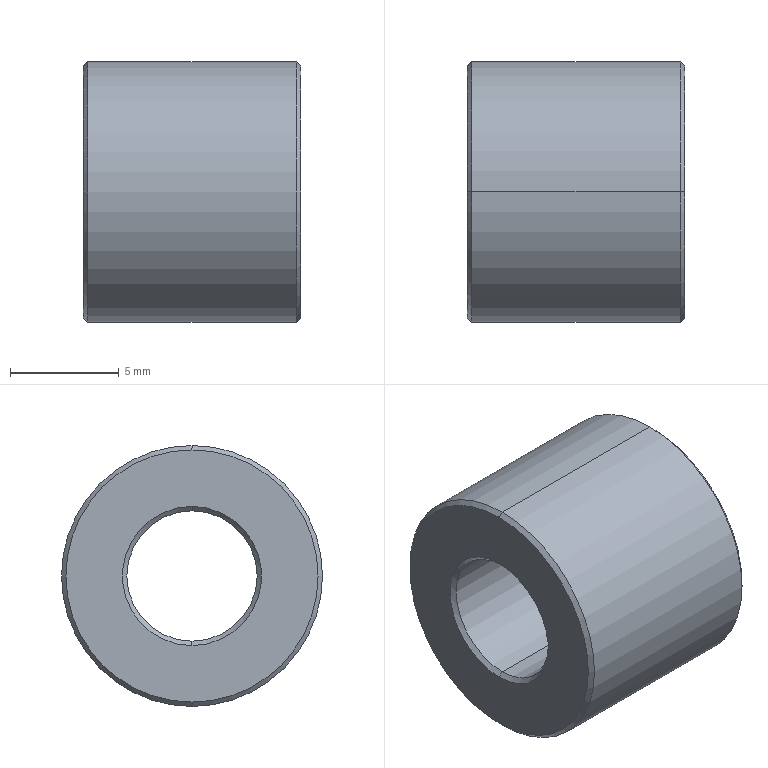Part | STEP file | KNCLM6-12-10 | 1 solid | 14 faces | box 10 x 12 x 12 mm | volume 845.968 mm3 | cone 8 | cylinder 4 | plane 2 | commonest cylinder face diameters 6 x2 12 x2
STEP:
#1=CARTESIAN_POINT('',(0.,0.,0.));
#2=DIRECTION('',(0.,0.,1.));
#3=DIRECTION('',(1.,0.,0.));
#4=AXIS2_PLACEMENT_3D('',#1,#2,#3);
#5=CARTESIAN_POINT('',(10.,0.,-5.8));
#6=VERTEX_POINT('',#5);
#7=CARTESIAN_POINT('',(10.,0.,5.8));
#8=VERTEX_POINT('',#7);
#9=CARTESIAN_POINT('',(10.,0.,0.));
#10=DIRECTION('',(1.,0.,0.));
#11=DIRECTION('',(0.,0.,1.));
#12=AXIS2_PLACEMENT_3D('',#9,#10,#11);
#13=CIRCLE('',#12,5.8);
#14=CARTESIAN_POINT('',(9.8,0.,0.));
#15=DIRECTION('',(-1.,0.,0.));
#16=DIRECTION('',(0.,0.,1.));
#17=AXIS2_PLACEMENT_3D('',#14,#15,#16);
#18=CONICAL_SURFACE('',#17,6.,0.7854);
#19=CARTESIAN_POINT('',(6.283,-0.2));
#20=DIRECTION('',(-1.,0.));
#21=VECTOR('',#20,1.);
#22=LINE('',#19,#21);
#23=(GEOMETRIC_REPRESENTATION_CONTEXT(2)PARAMETRIC_REPRESENTATION_CONTEXT()REPRESENTATION_CONTEXT('',''));
#24=DEFINITIONAL_REPRESENTATION('',(#22),#23);
#25=PCURVE('',#18,#24);
#26=CARTESIAN_POINT('',(10.,3.,0.));
#27=DIRECTION('',(-1.,0.,0.));
#28=DIRECTION('',(0.,0.,1.));
#29=AXIS2_PLACEMENT_3D('',#26,#27,#28);
#30=PLANE('',#29);
#31=CARTESIAN_POINT('',(5.8,-3.));
#32=CARTESIAN_POINT('',(5.8,-13.046));
#33=CARTESIAN_POINT('',(-2.9,-8.023));
#34=CARTESIAN_POINT('',(-11.6,-3.));
#35=CARTESIAN_POINT('',(-2.9,2.023));
#36=CARTESIAN_POINT('',(5.8,7.046));
#37=CARTESIAN_POINT('',(5.8,-3.));
#38=(BOUNDED_CURVE()B_SPLINE_CURVE(2,(#31,#32,#33,#34,#35,#36,#37),.UNSPECIFIED.,.T.,.F.)B_SPLINE_CURVE_WITH_KNOTS((1,2,2,2,2,1),(-2.094,0.,2.094,4.189,6.283,8.378),.UNSPECIFIED.)CURVE()GEOMETRIC_REPRESENTATION_ITEM()RATIONAL_B_SPLINE_CURVE((1.,0.5,1.,0.5,1.,0.5,1.))REPRESENTATION_ITEM(''));
#39=(GEOMETRIC_REPRESENTATION_CONTEXT(2)PARAMETRIC_REPRESENTATION_CONTEXT()REPRESENTATION_CONTEXT('',''));
#40=DEFINITIONAL_REPRESENTATION('',(#38),#39);
#41=PCURVE('',#30,#40);
#42=SURFACE_CURVE('',#13,(#25,#41),.PCURVE_S1.);
#43=EDGE_CURVE('',#6,#8,#42,.T.);
#44=ORIENTED_EDGE('',*,*,#43,.F.);
#45=CARTESIAN_POINT('',(9.8,0.,-6.));
#46=VERTEX_POINT('',#45);
#47=CARTESIAN_POINT('',(9.8,0.,-6.));
#48=DIRECTION('',(-0.7071,0.,-0.7071));
#49=VECTOR('',#48,1.);
#50=LINE('',#47,#49);
#51=CARTESIAN_POINT('',(3.142,0.));
#52=DIRECTION('',(0.,1.));
#53=VECTOR('',#52,1.);
#54=LINE('',#51,#53);
#55=(GEOMETRIC_REPRESENTATION_CONTEXT(2)PARAMETRIC_REPRESENTATION_CONTEXT()REPRESENTATION_CONTEXT('',''));
#56=DEFINITIONAL_REPRESENTATION('',(#54),#55);
#57=PCURVE('',#18,#56);
#58=CARTESIAN_POINT('',(9.8,0.,0.));
#59=DIRECTION('',(-1.,0.,0.));
#60=DIRECTION('',(0.,0.,1.));
#61=AXIS2_PLACEMENT_3D('',#58,#59,#60);
#62=CONICAL_SURFACE('',#61,6.,0.7854);
#63=CARTESIAN_POINT('',(3.142,0.));
#64=DIRECTION('',(0.,1.));
#65=VECTOR('',#64,1.);
#66=LINE('',#63,#65);
#67=(GEOMETRIC_REPRESENTATION_CONTEXT(2)PARAMETRIC_REPRESENTATION_CONTEXT()REPRESENTATION_CONTEXT('',''));
#68=DEFINITIONAL_REPRESENTATION('',(#66),#67);
#69=PCURVE('',#62,#68);
#70=SURFACE_CURVE('',#50,(#57,#69),.PCURVE_S1.);
#71=EDGE_CURVE('',#6,#46,#70,.T.);
#72=ORIENTED_EDGE('',*,*,#71,.T.);
#73=CARTESIAN_POINT('',(9.8,0.,6.));
#74=VERTEX_POINT('',#73);
#75=CARTESIAN_POINT('',(9.8,0.,0.));
#76=DIRECTION('',(-1.,0.,0.));
#77=DIRECTION('',(0.,0.,1.));
#78=AXIS2_PLACEMENT_3D('',#75,#76,#77);
#79=CIRCLE('',#78,6.);
#80=CARTESIAN_POINT('',(0.,0.));
#81=DIRECTION('',(1.,0.));
#82=VECTOR('',#81,1.);
#83=LINE('',#80,#82);
#84=(GEOMETRIC_REPRESENTATION_CONTEXT(2)PARAMETRIC_REPRESENTATION_CONTEXT()REPRESENTATION_CONTEXT('',''));
#85=DEFINITIONAL_REPRESENTATION('',(#83),#84);
#86=PCURVE('',#18,#85);
#87=CARTESIAN_POINT('',(0.,0.,0.));
#88=DIRECTION('',(-1.,0.,0.));
#89=DIRECTION('',(0.,0.,1.));
#90=AXIS2_PLACEMENT_3D('',#87,#88,#89);
#91=CYLINDRICAL_SURFACE('',#90,6.);
#92=CARTESIAN_POINT('',(0.,-9.8));
#93=DIRECTION('',(1.,0.));
#94=VECTOR('',#93,1.);
#95=LINE('',#92,#94);
#96=(GEOMETRIC_REPRESENTATION_CONTEXT(2)PARAMETRIC_REPRESENTATION_CONTEXT()REPRESENTATION_CONTEXT('',''));
#97=DEFINITIONAL_REPRESENTATION('',(#95),#96);
#98=PCURVE('',#91,#97);
#99=SURFACE_CURVE('',#79,(#86,#98),.PCURVE_S1.);
#100=EDGE_CURVE('',#74,#46,#99,.T.);
#101=ORIENTED_EDGE('',*,*,#100,.F.);
#102=CARTESIAN_POINT('',(9.8,0.,6.));
#103=DIRECTION('',(-0.7071,0.,0.7071));
#104=VECTOR('',#103,1.);
#105=LINE('',#102,#104);
#106=CARTESIAN_POINT('',(0.,0.));
#107=DIRECTION('',(0.,1.));
#108=VECTOR('',#107,1.);
#109=LINE('',#106,#108);
#110=(GEOMETRIC_REPRESENTATION_CONTEXT(2)PARAMETRIC_REPRESENTATION_CONTEXT()REPRESENTATION_CONTEXT('',''));
#111=DEFINITIONAL_REPRESENTATION('',(#109),#110);
#112=PCURVE('',#18,#111);
#113=CARTESIAN_POINT('',(6.283,0.));
#114=DIRECTION('',(0.,1.));
#115=VECTOR('',#114,1.);
#116=LINE('',#113,#115);
#117=(GEOMETRIC_REPRESENTATION_CONTEXT(2)PARAMETRIC_REPRESENTATION_CONTEXT()REPRESENTATION_CONTEXT('',''));
#118=DEFINITIONAL_REPRESENTATION('',(#116),#117);
#119=PCURVE('',#62,#118);
#120=SURFACE_CURVE('',#105,(#112,#119),.PCURVE_S1.);
#121=EDGE_CURVE('',#8,#74,#120,.T.);
#122=ORIENTED_EDGE('',*,*,#121,.F.);
#123=EDGE_LOOP('',(#44,#72,#101,#122));
#124=FACE_BOUND('',#123,.T.);
#125=ADVANCED_FACE('',(#124),#18,.T.);
#126=CARTESIAN_POINT('',(9.8,0.,-3.));
#127=VERTEX_POINT('',#126);
#128=CARTESIAN_POINT('',(10.,0.,-3.2));
#129=VERTEX_POINT('',#128);
#130=CARTESIAN_POINT('',(10.,0.,-3.2));
#131=DIRECTION('',(0.7071,0.,-0.7071));
#132=VECTOR('',#131,1.);
#133=LINE('',#130,#132);
#134=CARTESIAN_POINT('',(10.,0.,0.));
#135=DIRECTION('',(1.,0.,0.));
#136=DIRECTION('',(0.,0.,-1.));
#137=AXIS2_PLACEMENT_3D('',#134,#135,#136);
#138=CONICAL_SURFACE('',#137,3.2,0.7854);
#139=CARTESIAN_POINT('',(6.283,0.));
#140=DIRECTION('',(0.,1.));
#141=VECTOR('',#140,1.);
#142=LINE('',#139,#141);
#143=(GEOMETRIC_REPRESENTATION_CONTEXT(2)PARAMETRIC_REPRESENTATION_CONTEXT()REPRESENTATION_CONTEXT('',''));
#144=DEFINITIONAL_REPRESENTATION('',(#142),#143);
#145=PCURVE('',#138,#144);
#146=CARTESIAN_POINT('',(10.,0.,0.));
#147=DIRECTION('',(1.,0.,0.));
#148=DIRECTION('',(0.,0.,-1.));
#149=AXIS2_PLACEMENT_3D('',#146,#147,#148);
#150=CONICAL_SURFACE('',#149,3.2,0.7854);
#151=CARTESIAN_POINT('',(0.,0.));
#152=DIRECTION('',(0.,1.));
#153=VECTOR('',#152,1.);
#154=LINE('',#151,#153);
#155=(GEOMETRIC_REPRESENTATION_CONTEXT(2)PARAMETRIC_REPRESENTATION_CONTEXT()REPRESENTATION_CONTEXT('',''));
#156=DEFINITIONAL_REPRESENTATION('',(#154),#155);
#157=PCURVE('',#150,#156);
#158=SURFACE_CURVE('',#133,(#145,#157),.PCURVE_S1.);
#159=EDGE_CURVE('',#127,#129,#158,.T.);
#160=ORIENTED_EDGE('',*,*,#159,.T.);
#161=CARTESIAN_POINT('',(10.,0.,3.2));
#162=VERTEX_POINT('',#161);
#163=CARTESIAN_POINT('',(10.,0.,0.));
#164=DIRECTION('',(-1.,0.,0.));
#165=DIRECTION('',(0.,0.,1.));
#166=AXIS2_PLACEMENT_3D('',#163,#164,#165);
#167=CIRCLE('',#166,3.2);
#168=CARTESIAN_POINT('',(9.425,0.));
#169=DIRECTION('',(-1.,0.));
#170=VECTOR('',#169,1.);
#171=LINE('',#168,#170);
#172=(GEOMETRIC_REPRESENTATION_CONTEXT(2)PARAMETRIC_REPRESENTATION_CONTEXT()REPRESENTATION_CONTEXT('',''));
#173=DEFINITIONAL_REPRESENTATION('',(#171),#172);
#174=PCURVE('',#138,#173);
#175=CARTESIAN_POINT('',(0.,-3.));
#176=DIRECTION('',(1.,0.));
#177=AXIS2_PLACEMENT_2D('',#175,#176);
#178=CIRCLE('',#177,3.2);
#179=(GEOMETRIC_REPRESENTATION_CONTEXT(2)PARAMETRIC_REPRESENTATION_CONTEXT()REPRESENTATION_CONTEXT('',''));
#180=DEFINITIONAL_REPRESENTATION('',(#178),#179);
#181=PCURVE('',#30,#180);
#182=SURFACE_CURVE('',#167,(#174,#181),.PCURVE_S1.);
#183=EDGE_CURVE('',#129,#162,#182,.T.);
#184=ORIENTED_EDGE('',*,*,#183,.T.);
#185=CARTESIAN_POINT('',(9.8,0.,3.));
#186=VERTEX_POINT('',#185);
#187=CARTESIAN_POINT('',(10.,0.,3.2));
#188=DIRECTION('',(0.7071,0.,0.7071));
#189=VECTOR('',#188,1.);
#190=LINE('',#187,#189);
#191=CARTESIAN_POINT('',(3.142,0.));
#192=DIRECTION('',(0.,1.));
#193=VECTOR('',#192,1.);
#194=LINE('',#191,#193);
#195=(GEOMETRIC_REPRESENTATION_CONTEXT(2)PARAMETRIC_REPRESENTATION_CONTEXT()REPRESENTATION_CONTEXT('',''));
#196=DEFINITIONAL_REPRESENTATION('',(#194),#195);
#197=PCURVE('',#138,#196);
#198=CARTESIAN_POINT('',(3.142,0.));
#199=DIRECTION('',(0.,1.));
#200=VECTOR('',#199,1.);
#201=LINE('',#198,#200);
#202=(GEOMETRIC_REPRESENTATION_CONTEXT(2)PARAMETRIC_REPRESENTATION_CONTEXT()REPRESENTATION_CONTEXT('',''));
#203=DEFINITIONAL_REPRESENTATION('',(#201),#202);
#204=PCURVE('',#150,#203);
#205=SURFACE_CURVE('',#190,(#197,#204),.PCURVE_S1.);
#206=EDGE_CURVE('',#186,#162,#205,.T.);
#207=ORIENTED_EDGE('',*,*,#206,.F.);
#208=CARTESIAN_POINT('',(9.8,0.,0.));
#209=DIRECTION('',(1.,0.,0.));
#210=DIRECTION('',(0.,0.,1.));
#211=AXIS2_PLACEMENT_3D('',#208,#209,#210);
#212=CIRCLE('',#211,3.);
#213=CARTESIAN_POINT('',(3.142,-0.2));
#214=DIRECTION('',(1.,0.));
#215=VECTOR('',#214,1.);
#216=LINE('',#213,#215);
#217=(GEOMETRIC_REPRESENTATION_CONTEXT(2)PARAMETRIC_REPRESENTATION_CONTEXT()REPRESENTATION_CONTEXT('',''));
#218=DEFINITIONAL_REPRESENTATION('',(#216),#217);
#219=PCURVE('',#138,#218);
#220=CARTESIAN_POINT('',(0.,0.,0.));
#221=DIRECTION('',(-1.,0.,0.));
#222=DIRECTION('',(0.,0.,1.));
#223=AXIS2_PLACEMENT_3D('',#220,#221,#222);
#224=CYLINDRICAL_SURFACE('',#223,3.);
#225=CARTESIAN_POINT('',(6.283,-9.8));
#226=DIRECTION('',(-1.,0.));
#227=VECTOR('',#226,1.);
#228=LINE('',#225,#227);
#229=(GEOMETRIC_REPRESENTATION_CONTEXT(2)PARAMETRIC_REPRESENTATION_CONTEXT()REPRESENTATION_CONTEXT('',''));
#230=DEFINITIONAL_REPRESENTATION('',(#228),#229);
#231=PCURVE('',#224,#230);
#232=SURFACE_CURVE('',#212,(#219,#231),.PCURVE_S1.);
#233=EDGE_CURVE('',#186,#127,#232,.T.);
#234=ORIENTED_EDGE('',*,*,#233,.T.);
#235=EDGE_LOOP('',(#160,#184,#207,#234));
#236=FACE_BOUND('',#235,.F.);
#237=ADVANCED_FACE('',(#236),#138,.F.);
#238=CARTESIAN_POINT('',(0.,0.,5.8));
#239=VERTEX_POINT('',#238);
#240=CARTESIAN_POINT('',(0.,0.,-5.8));
#241=VERTEX_POINT('',#240);
#242=CARTESIAN_POINT('',(0.,0.,0.));
#243=DIRECTION('',(-1.,0.,0.));
#244=DIRECTION('',(0.,0.,-1.));
#245=AXIS2_PLACEMENT_3D('',#242,#243,#244);
#246=CIRCLE('',#245,5.8);
#247=CARTESIAN_POINT('',(0.,0.,0.));
#248=DIRECTION('',(1.,0.,0.));
#249=DIRECTION('',(0.,0.,-1.));
#250=AXIS2_PLACEMENT_3D('',#247,#248,#249);
#251=CONICAL_SURFACE('',#250,5.8,0.7854);
#252=CARTESIAN_POINT('',(6.283,0.));
#253=DIRECTION('',(-1.,0.));
#254=VECTOR('',#253,1.);
#255=LINE('',#252,#254);
#256=(GEOMETRIC_REPRESENTATION_CONTEXT(2)PARAMETRIC_REPRESENTATION_CONTEXT()REPRESENTATION_CONTEXT('',''));
#257=DEFINITIONAL_REPRESENTATION('',(#255),#256);
#258=PCURVE('',#251,#257);
#259=CARTESIAN_POINT('',(0.,3.,0.));
#260=DIRECTION('',(1.,0.,0.));
#261=DIRECTION('',(0.,0.,-1.));
#262=AXIS2_PLACEMENT_3D('',#259,#260,#261);
#263=PLANE('',#262);
#264=CARTESIAN_POINT('',(5.8,-3.));
#265=CARTESIAN_POINT('',(5.8,-13.046));
#266=CARTESIAN_POINT('',(-2.9,-8.023));
#267=CARTESIAN_POINT('',(-11.6,-3.));
#268=CARTESIAN_POINT('',(-2.9,2.023));
#269=CARTESIAN_POINT('',(5.8,7.046));
#270=CARTESIAN_POINT('',(5.8,-3.));
#271=(BOUNDED_CURVE()B_SPLINE_CURVE(2,(#264,#265,#266,#267,#268,#269,#270),.UNSPECIFIED.,.T.,.F.)B_SPLINE_CURVE_WITH_KNOTS((1,2,2,2,2,1),(-2.094,0.,2.094,4.189,6.283,8.378),.UNSPECIFIED.)CURVE()GEOMETRIC_REPRESENTATION_ITEM()RATIONAL_B_SPLINE_CURVE((1.,0.5,1.,0.5,1.,0.5,1.))REPRESENTATION_ITEM(''));
#272=(GEOMETRIC_REPRESENTATION_CONTEXT(2)PARAMETRIC_REPRESENTATION_CONTEXT()REPRESENTATION_CONTEXT('',''));
#273=DEFINITIONAL_REPRESENTATION('',(#271),#272);
#274=PCURVE('',#263,#273);
#275=SURFACE_CURVE('',#246,(#258,#274),.PCURVE_S1.);
#276=EDGE_CURVE('',#239,#241,#275,.T.);
#277=ORIENTED_EDGE('',*,*,#276,.F.);
#278=CARTESIAN_POINT('',(0.2,0.,6.));
#279=VERTEX_POINT('',#278);
#280=CARTESIAN_POINT('',(0.,0.,5.8));
#281=DIRECTION('',(0.7071,0.,0.7071));
#282=VECTOR('',#281,1.);
#283=LINE('',#280,#282);
#284=CARTESIAN_POINT('',(3.142,0.));
#285=DIRECTION('',(0.,1.));
#286=VECTOR('',#285,1.);
#287=LINE('',#284,#286);
#288=(GEOMETRIC_REPRESENTATION_CONTEXT(2)PARAMETRIC_REPRESENTATION_CONTEXT()REPRESENTATION_CONTEXT('',''));
#289=DEFINITIONAL_REPRESENTATION('',(#287),#288);
#290=PCURVE('',#251,#289);
#291=CARTESIAN_POINT('',(0.,0.,0.));
#292=DIRECTION('',(1.,0.,0.));
#293=DIRECTION('',(0.,0.,-1.));
#294=AXIS2_PLACEMENT_3D('',#291,#292,#293);
#295=CONICAL_SURFACE('',#294,5.8,0.7854);
#296=CARTESIAN_POINT('',(3.142,0.));
#297=DIRECTION('',(0.,1.));
#298=VECTOR('',#297,1.);
#299=LINE('',#296,#298);
#300=(GEOMETRIC_REPRESENTATION_CONTEXT(2)PARAMETRIC_REPRESENTATION_CONTEXT()REPRESENTATION_CONTEXT('',''));
#301=DEFINITIONAL_REPRESENTATION('',(#299),#300);
#302=PCURVE('',#295,#301);
#303=SURFACE_CURVE('',#283,(#290,#302),.PCURVE_S1.);
#304=EDGE_CURVE('',#239,#279,#303,.T.);
#305=ORIENTED_EDGE('',*,*,#304,.T.);
#306=CARTESIAN_POINT('',(0.2,0.,-6.));
#307=VERTEX_POINT('',#306);
#308=CARTESIAN_POINT('',(0.2,0.,0.));
#309=DIRECTION('',(1.,0.,0.));
#310=DIRECTION('',(0.,0.,-1.));
#311=AXIS2_PLACEMENT_3D('',#308,#309,#310);
#312=CIRCLE('',#311,6.);
#313=CARTESIAN_POINT('',(0.,0.2));
#314=DIRECTION('',(1.,0.));
#315=VECTOR('',#314,1.);
#316=LINE('',#313,#315);
#317=(GEOMETRIC_REPRESENTATION_CONTEXT(2)PARAMETRIC_REPRESENTATION_CONTEXT()REPRESENTATION_CONTEXT('',''));
#318=DEFINITIONAL_REPRESENTATION('',(#316),#317);
#319=PCURVE('',#251,#318);
#320=CARTESIAN_POINT('',(3.142,-0.2));
#321=DIRECTION('',(-1.,0.));
#322=VECTOR('',#321,1.);
#323=LINE('',#320,#322);
#324=(GEOMETRIC_REPRESENTATION_CONTEXT(2)PARAMETRIC_REPRESENTATION_CONTEXT()REPRESENTATION_CONTEXT('',''));
#325=DEFINITIONAL_REPRESENTATION('',(#323),#324);
#326=PCURVE('',#91,#325);
#327=SURFACE_CURVE('',#312,(#319,#326),.PCURVE_S1.);
#328=EDGE_CURVE('',#307,#279,#327,.T.);
#329=ORIENTED_EDGE('',*,*,#328,.F.);
#330=CARTESIAN_POINT('',(0.,0.,-5.8));
#331=DIRECTION('',(0.7071,0.,-0.7071));
#332=VECTOR('',#331,1.);
#333=LINE('',#330,#332);
#334=CARTESIAN_POINT('',(0.,0.));
#335=DIRECTION('',(0.,1.));
#336=VECTOR('',#335,1.);
#337=LINE('',#334,#336);
#338=(GEOMETRIC_REPRESENTATION_CONTEXT(2)PARAMETRIC_REPRESENTATION_CONTEXT()REPRESENTATION_CONTEXT('',''));
#339=DEFINITIONAL_REPRESENTATION('',(#337),#338);
#340=PCURVE('',#251,#339);
#341=CARTESIAN_POINT('',(6.283,0.));
#342=DIRECTION('',(0.,1.));
#343=VECTOR('',#342,1.);
#344=LINE('',#341,#343);
#345=(GEOMETRIC_REPRESENTATION_CONTEXT(2)PARAMETRIC_REPRESENTATION_CONTEXT()REPRESENTATION_CONTEXT('',''));
#346=DEFINITIONAL_REPRESENTATION('',(#344),#345);
#347=PCURVE('',#295,#346);
#348=SURFACE_CURVE('',#333,(#340,#347),.PCURVE_S1.);
#349=EDGE_CURVE('',#241,#307,#348,.T.);
#350=ORIENTED_EDGE('',*,*,#349,.F.);
#351=EDGE_LOOP('',(#277,#305,#329,#350));
#352=FACE_BOUND('',#351,.T.);
#353=ADVANCED_FACE('',(#352),#251,.T.);
#354=CARTESIAN_POINT('',(0.2,0.,3.));
#355=VERTEX_POINT('',#354);
#356=CARTESIAN_POINT('',(0.,0.,3.2));
#357=VERTEX_POINT('',#356);
#358=CARTESIAN_POINT('',(0.2,0.,3.));
#359=DIRECTION('',(-0.7071,0.,0.7071));
#360=VECTOR('',#359,1.);
#361=LINE('',#358,#360);
#362=CARTESIAN_POINT('',(0.2,0.,0.));
#363=DIRECTION('',(-1.,0.,0.));
#364=DIRECTION('',(0.,0.,1.));
#365=AXIS2_PLACEMENT_3D('',#362,#363,#364);
#366=CONICAL_SURFACE('',#365,3.,0.7854);
#367=CARTESIAN_POINT('',(6.283,0.));
#368=DIRECTION('',(0.,1.));
#369=VECTOR('',#368,1.);
#370=LINE('',#367,#369);
#371=(GEOMETRIC_REPRESENTATION_CONTEXT(2)PARAMETRIC_REPRESENTATION_CONTEXT()REPRESENTATION_CONTEXT('',''));
#372=DEFINITIONAL_REPRESENTATION('',(#370),#371);
#373=PCURVE('',#366,#372);
#374=CARTESIAN_POINT('',(0.2,0.,0.));
#375=DIRECTION('',(-1.,0.,0.));
#376=DIRECTION('',(0.,0.,1.));
#377=AXIS2_PLACEMENT_3D('',#374,#375,#376);
#378=CONICAL_SURFACE('',#377,3.,0.7854);
#379=CARTESIAN_POINT('',(0.,0.));
#380=DIRECTION('',(0.,1.));
#381=VECTOR('',#380,1.);
#382=LINE('',#379,#381);
#383=(GEOMETRIC_REPRESENTATION_CONTEXT(2)PARAMETRIC_REPRESENTATION_CONTEXT()REPRESENTATION_CONTEXT('',''));
#384=DEFINITIONAL_REPRESENTATION('',(#382),#383);
#385=PCURVE('',#378,#384);
#386=SURFACE_CURVE('',#361,(#373,#385),.PCURVE_S1.);
#387=EDGE_CURVE('',#355,#357,#386,.T.);
#388=ORIENTED_EDGE('',*,*,#387,.T.);
#389=CARTESIAN_POINT('',(0.,0.,-3.2));
#390=VERTEX_POINT('',#389);
#391=CARTESIAN_POINT('',(0.,0.,0.));
#392=DIRECTION('',(1.,0.,0.));
#393=DIRECTION('',(0.,0.,-1.));
#394=AXIS2_PLACEMENT_3D('',#391,#392,#393);
#395=CIRCLE('',#394,3.2);
#396=CARTESIAN_POINT('',(9.425,0.2));
#397=DIRECTION('',(-1.,0.));
#398=VECTOR('',#397,1.);
#399=LINE('',#396,#398);
#400=(GEOMETRIC_REPRESENTATION_CONTEXT(2)PARAMETRIC_REPRESENTATION_CONTEXT()REPRESENTATION_CONTEXT('',''));
#401=DEFINITIONAL_REPRESENTATION('',(#399),#400);
#402=PCURVE('',#366,#401);
#403=CARTESIAN_POINT('',(0.,-3.));
#404=DIRECTION('',(1.,0.));
#405=AXIS2_PLACEMENT_2D('',#403,#404);
#406=CIRCLE('',#405,3.2);
#407=(GEOMETRIC_REPRESENTATION_CONTEXT(2)PARAMETRIC_REPRESENTATION_CONTEXT()REPRESENTATION_CONTEXT('',''));
#408=DEFINITIONAL_REPRESENTATION('',(#406),#407);
#409=PCURVE('',#263,#408);
#410=SURFACE_CURVE('',#395,(#402,#409),.PCURVE_S1.);
#411=EDGE_CURVE('',#357,#390,#410,.T.);
#412=ORIENTED_EDGE('',*,*,#411,.T.);
#413=CARTESIAN_POINT('',(0.2,0.,-3.));
#414=VERTEX_POINT('',#413);
#415=CARTESIAN_POINT('',(0.2,0.,-3.));
#416=DIRECTION('',(-0.7071,0.,-0.7071));
#417=VECTOR('',#416,1.);
#418=LINE('',#415,#417);
#419=CARTESIAN_POINT('',(3.142,0.));
#420=DIRECTION('',(0.,1.));
#421=VECTOR('',#420,1.);
#422=LINE('',#419,#421);
#423=(GEOMETRIC_REPRESENTATION_CONTEXT(2)PARAMETRIC_REPRESENTATION_CONTEXT()REPRESENTATION_CONTEXT('',''));
#424=DEFINITIONAL_REPRESENTATION('',(#422),#423);
#425=PCURVE('',#366,#424);
#426=CARTESIAN_POINT('',(3.142,0.));
#427=DIRECTION('',(0.,1.));
#428=VECTOR('',#427,1.);
#429=LINE('',#426,#428);
#430=(GEOMETRIC_REPRESENTATION_CONTEXT(2)PARAMETRIC_REPRESENTATION_CONTEXT()REPRESENTATION_CONTEXT('',''));
#431=DEFINITIONAL_REPRESENTATION('',(#429),#430);
#432=PCURVE('',#378,#431);
#433=SURFACE_CURVE('',#418,(#425,#432),.PCURVE_S1.);
#434=EDGE_CURVE('',#414,#390,#433,.T.);
#435=ORIENTED_EDGE('',*,*,#434,.F.);
#436=CARTESIAN_POINT('',(0.2,0.,0.));
#437=DIRECTION('',(-1.,0.,0.));
#438=DIRECTION('',(0.,0.,-1.));
#439=AXIS2_PLACEMENT_3D('',#436,#437,#438);
#440=CIRCLE('',#439,3.);
#441=CARTESIAN_POINT('',(3.142,0.));
#442=DIRECTION('',(1.,0.));
#443=VECTOR('',#442,1.);
#444=LINE('',#441,#443);
#445=(GEOMETRIC_REPRESENTATION_CONTEXT(2)PARAMETRIC_REPRESENTATION_CONTEXT()REPRESENTATION_CONTEXT('',''));
#446=DEFINITIONAL_REPRESENTATION('',(#444),#445);
#447=PCURVE('',#366,#446);
#448=CARTESIAN_POINT('',(3.142,-0.2));
#449=DIRECTION('',(1.,0.));
#450=VECTOR('',#449,1.);
#451=LINE('',#448,#450);
#452=(GEOMETRIC_REPRESENTATION_CONTEXT(2)PARAMETRIC_REPRESENTATION_CONTEXT()REPRESENTATION_CONTEXT('',''));
#453=DEFINITIONAL_REPRESENTATION('',(#451),#452);
#454=PCURVE('',#224,#453);
#455=SURFACE_CURVE('',#440,(#447,#454),.PCURVE_S1.);
#456=EDGE_CURVE('',#414,#355,#455,.T.);
#457=ORIENTED_EDGE('',*,*,#456,.T.);
#458=EDGE_LOOP('',(#388,#412,#435,#457));
#459=FACE_BOUND('',#458,.F.);
#460=ADVANCED_FACE('',(#459),#366,.F.);
#461=CARTESIAN_POINT('',(0.,0.,3.));
#462=DIRECTION('',(-1.,0.,0.));
#463=VECTOR('',#462,1.);
#464=LINE('',#461,#463);
#465=CARTESIAN_POINT('',(6.283,0.));
#466=DIRECTION('',(0.,1.));
#467=VECTOR('',#466,1.);
#468=LINE('',#465,#467);
#469=(GEOMETRIC_REPRESENTATION_CONTEXT(2)PARAMETRIC_REPRESENTATION_CONTEXT()REPRESENTATION_CONTEXT('',''));
#470=DEFINITIONAL_REPRESENTATION('',(#468),#469);
#471=PCURVE('',#224,#470);
#472=CARTESIAN_POINT('',(0.,0.,0.));
#473=DIRECTION('',(-1.,0.,0.));
#474=DIRECTION('',(0.,0.,1.));
#475=AXIS2_PLACEMENT_3D('',#472,#473,#474);
#476=CYLINDRICAL_SURFACE('',#475,3.);
#477=CARTESIAN_POINT('',(0.,0.));
#478=DIRECTION('',(0.,1.));
#479=VECTOR('',#478,1.);
#480=LINE('',#477,#479);
#481=(GEOMETRIC_REPRESENTATION_CONTEXT(2)PARAMETRIC_REPRESENTATION_CONTEXT()REPRESENTATION_CONTEXT('',''));
#482=DEFINITIONAL_REPRESENTATION('',(#480),#481);
#483=PCURVE('',#476,#482);
#484=SURFACE_CURVE('',#464,(#471,#483),.PCURVE_S1.);
#485=EDGE_CURVE('',#186,#355,#484,.T.);
#486=ORIENTED_EDGE('',*,*,#485,.T.);
#487=ORIENTED_EDGE('',*,*,#456,.F.);
#488=CARTESIAN_POINT('',(0.,0.,-3.));
#489=DIRECTION('',(-1.,0.,0.));
#490=VECTOR('',#489,1.);
#491=LINE('',#488,#490);
#492=CARTESIAN_POINT('',(3.142,0.));
#493=DIRECTION('',(0.,1.));
#494=VECTOR('',#493,1.);
#495=LINE('',#492,#494);
#496=(GEOMETRIC_REPRESENTATION_CONTEXT(2)PARAMETRIC_REPRESENTATION_CONTEXT()REPRESENTATION_CONTEXT('',''));
#497=DEFINITIONAL_REPRESENTATION('',(#495),#496);
#498=PCURVE('',#224,#497);
#499=CARTESIAN_POINT('',(3.142,0.));
#500=DIRECTION('',(0.,1.));
#501=VECTOR('',#500,1.);
#502=LINE('',#499,#501);
#503=(GEOMETRIC_REPRESENTATION_CONTEXT(2)PARAMETRIC_REPRESENTATION_CONTEXT()REPRESENTATION_CONTEXT('',''));
#504=DEFINITIONAL_REPRESENTATION('',(#502),#503);
#505=PCURVE('',#476,#504);
#506=SURFACE_CURVE('',#491,(#498,#505),.PCURVE_S1.);
#507=EDGE_CURVE('',#127,#414,#506,.T.);
#508=ORIENTED_EDGE('',*,*,#507,.F.);
#509=ORIENTED_EDGE('',*,*,#233,.F.);
#510=EDGE_LOOP('',(#486,#487,#508,#509));
#511=FACE_BOUND('',#510,.F.);
#512=ADVANCED_FACE('',(#511),#224,.F.);
#513=ORIENTED_EDGE('',*,*,#100,.T.);
#514=CARTESIAN_POINT('',(0.,0.,-6.));
#515=DIRECTION('',(-1.,0.,0.));
#516=VECTOR('',#515,1.);
#517=LINE('',#514,#516);
#518=CARTESIAN_POINT('',(3.142,0.));
#519=DIRECTION('',(0.,1.));
#520=VECTOR('',#519,1.);
#521=LINE('',#518,#520);
#522=(GEOMETRIC_REPRESENTATION_CONTEXT(2)PARAMETRIC_REPRESENTATION_CONTEXT()REPRESENTATION_CONTEXT('',''));
#523=DEFINITIONAL_REPRESENTATION('',(#521),#522);
#524=PCURVE('',#91,#523);
#525=CARTESIAN_POINT('',(0.,0.,0.));
#526=DIRECTION('',(-1.,0.,0.));
#527=DIRECTION('',(0.,0.,1.));
#528=AXIS2_PLACEMENT_3D('',#525,#526,#527);
#529=CYLINDRICAL_SURFACE('',#528,6.);
#530=CARTESIAN_POINT('',(3.142,0.));
#531=DIRECTION('',(0.,1.));
#532=VECTOR('',#531,1.);
#533=LINE('',#530,#532);
#534=(GEOMETRIC_REPRESENTATION_CONTEXT(2)PARAMETRIC_REPRESENTATION_CONTEXT()REPRESENTATION_CONTEXT('',''));
#535=DEFINITIONAL_REPRESENTATION('',(#533),#534);
#536=PCURVE('',#529,#535);
#537=SURFACE_CURVE('',#517,(#524,#536),.PCURVE_S1.);
#538=EDGE_CURVE('',#46,#307,#537,.T.);
#539=ORIENTED_EDGE('',*,*,#538,.T.);
#540=ORIENTED_EDGE('',*,*,#328,.T.);
#541=CARTESIAN_POINT('',(0.,0.,6.));
#542=DIRECTION('',(-1.,0.,0.));
#543=VECTOR('',#542,1.);
#544=LINE('',#541,#543);
#545=CARTESIAN_POINT('',(0.,0.));
#546=DIRECTION('',(0.,1.));
#547=VECTOR('',#546,1.);
#548=LINE('',#545,#547);
#549=(GEOMETRIC_REPRESENTATION_CONTEXT(2)PARAMETRIC_REPRESENTATION_CONTEXT()REPRESENTATION_CONTEXT('',''));
#550=DEFINITIONAL_REPRESENTATION('',(#548),#549);
#551=PCURVE('',#91,#550);
#552=CARTESIAN_POINT('',(6.283,0.));
#553=DIRECTION('',(0.,1.));
#554=VECTOR('',#553,1.);
#555=LINE('',#552,#554);
#556=(GEOMETRIC_REPRESENTATION_CONTEXT(2)PARAMETRIC_REPRESENTATION_CONTEXT()REPRESENTATION_CONTEXT('',''));
#557=DEFINITIONAL_REPRESENTATION('',(#555),#556);
#558=PCURVE('',#529,#557);
#559=SURFACE_CURVE('',#544,(#551,#558),.PCURVE_S1.);
#560=EDGE_CURVE('',#74,#279,#559,.T.);
#561=ORIENTED_EDGE('',*,*,#560,.F.);
#562=EDGE_LOOP('',(#513,#539,#540,#561));
#563=FACE_BOUND('',#562,.T.);
#564=ADVANCED_FACE('',(#563),#91,.T.);
#565=ORIENTED_EDGE('',*,*,#411,.T.);
#566=CARTESIAN_POINT('',(0.,0.,0.));
#567=DIRECTION('',(1.,0.,0.));
#568=DIRECTION('',(0.,0.,-1.));
#569=AXIS2_PLACEMENT_3D('',#566,#567,#568);
#570=CIRCLE('',#569,3.2);
#571=CARTESIAN_POINT('',(0.,-3.));
#572=DIRECTION('',(1.,0.));
#573=AXIS2_PLACEMENT_2D('',#571,#572);
#574=CIRCLE('',#573,3.2);
#575=(GEOMETRIC_REPRESENTATION_CONTEXT(2)PARAMETRIC_REPRESENTATION_CONTEXT()REPRESENTATION_CONTEXT('',''));
#576=DEFINITIONAL_REPRESENTATION('',(#574),#575);
#577=PCURVE('',#263,#576);
#578=CARTESIAN_POINT('',(3.142,0.2));
#579=DIRECTION('',(-1.,0.));
#580=VECTOR('',#579,1.);
#581=LINE('',#578,#580);
#582=(GEOMETRIC_REPRESENTATION_CONTEXT(2)PARAMETRIC_REPRESENTATION_CONTEXT()REPRESENTATION_CONTEXT('',''));
#583=DEFINITIONAL_REPRESENTATION('',(#581),#582);
#584=PCURVE('',#378,#583);
#585=SURFACE_CURVE('',#570,(#577,#584),.PCURVE_S1.);
#586=EDGE_CURVE('',#390,#357,#585,.T.);
#587=ORIENTED_EDGE('',*,*,#586,.T.);
#588=EDGE_LOOP('',(#565,#587));
#589=FACE_BOUND('',#588,.T.);
#590=CARTESIAN_POINT('',(0.,0.,0.));
#591=DIRECTION('',(-1.,0.,0.));
#592=DIRECTION('',(0.,0.,-1.));
#593=AXIS2_PLACEMENT_3D('',#590,#591,#592);
#594=CIRCLE('',#593,5.8);
#595=CARTESIAN_POINT('',(5.8,-3.));
#596=CARTESIAN_POINT('',(5.8,-13.046));
#597=CARTESIAN_POINT('',(-2.9,-8.023));
#598=CARTESIAN_POINT('',(-11.6,-3.));
#599=CARTESIAN_POINT('',(-2.9,2.023));
#600=CARTESIAN_POINT('',(5.8,7.046));
#601=CARTESIAN_POINT('',(5.8,-3.));
#602=(BOUNDED_CURVE()B_SPLINE_CURVE(2,(#595,#596,#597,#598,#599,#600,#601),.UNSPECIFIED.,.T.,.F.)B_SPLINE_CURVE_WITH_KNOTS((1,2,2,2,2,1),(-2.094,0.,2.094,4.189,6.283,8.378),.UNSPECIFIED.)CURVE()GEOMETRIC_REPRESENTATION_ITEM()RATIONAL_B_SPLINE_CURVE((1.,0.5,1.,0.5,1.,0.5,1.))REPRESENTATION_ITEM(''));
#603=(GEOMETRIC_REPRESENTATION_CONTEXT(2)PARAMETRIC_REPRESENTATION_CONTEXT()REPRESENTATION_CONTEXT('',''));
#604=DEFINITIONAL_REPRESENTATION('',(#602),#603);
#605=PCURVE('',#263,#604);
#606=CARTESIAN_POINT('',(6.283,0.));
#607=DIRECTION('',(-1.,0.));
#608=VECTOR('',#607,1.);
#609=LINE('',#606,#608);
#610=(GEOMETRIC_REPRESENTATION_CONTEXT(2)PARAMETRIC_REPRESENTATION_CONTEXT()REPRESENTATION_CONTEXT('',''));
#611=DEFINITIONAL_REPRESENTATION('',(#609),#610);
#612=PCURVE('',#295,#611);
#613=SURFACE_CURVE('',#594,(#605,#612),.PCURVE_S1.);
#614=EDGE_CURVE('',#241,#239,#613,.T.);
#615=ORIENTED_EDGE('',*,*,#614,.T.);
#616=ORIENTED_EDGE('',*,*,#276,.T.);
#617=EDGE_LOOP('',(#615,#616));
#618=FACE_BOUND('',#617,.T.);
#619=ADVANCED_FACE('',(#589,#618),#263,.F.);
#620=ORIENTED_EDGE('',*,*,#538,.F.);
#621=CARTESIAN_POINT('',(9.8,0.,0.));
#622=DIRECTION('',(-1.,0.,0.));
#623=DIRECTION('',(0.,0.,1.));
#624=AXIS2_PLACEMENT_3D('',#621,#622,#623);
#625=CIRCLE('',#624,6.);
#626=CARTESIAN_POINT('',(0.,-9.8));
#627=DIRECTION('',(1.,0.));
#628=VECTOR('',#627,1.);
#629=LINE('',#626,#628);
#630=(GEOMETRIC_REPRESENTATION_CONTEXT(2)PARAMETRIC_REPRESENTATION_CONTEXT()REPRESENTATION_CONTEXT('',''));
#631=DEFINITIONAL_REPRESENTATION('',(#629),#630);
#632=PCURVE('',#529,#631);
#633=CARTESIAN_POINT('',(0.,0.));
#634=DIRECTION('',(1.,0.));
#635=VECTOR('',#634,1.);
#636=LINE('',#633,#635);
#637=(GEOMETRIC_REPRESENTATION_CONTEXT(2)PARAMETRIC_REPRESENTATION_CONTEXT()REPRESENTATION_CONTEXT('',''));
#638=DEFINITIONAL_REPRESENTATION('',(#636),#637);
#639=PCURVE('',#62,#638);
#640=SURFACE_CURVE('',#625,(#632,#639),.PCURVE_S1.);
#641=EDGE_CURVE('',#46,#74,#640,.T.);
#642=ORIENTED_EDGE('',*,*,#641,.T.);
#643=ORIENTED_EDGE('',*,*,#560,.T.);
#644=CARTESIAN_POINT('',(0.2,0.,0.));
#645=DIRECTION('',(1.,0.,0.));
#646=DIRECTION('',(0.,0.,-1.));
#647=AXIS2_PLACEMENT_3D('',#644,#645,#646);
#648=CIRCLE('',#647,6.);
#649=CARTESIAN_POINT('',(9.425,-0.2));
#650=DIRECTION('',(-1.,0.));
#651=VECTOR('',#650,1.);
#652=LINE('',#649,#651);
#653=(GEOMETRIC_REPRESENTATION_CONTEXT(2)PARAMETRIC_REPRESENTATION_CONTEXT()REPRESENTATION_CONTEXT('',''));
#654=DEFINITIONAL_REPRESENTATION('',(#652),#653);
#655=PCURVE('',#529,#654);
#656=CARTESIAN_POINT('',(0.,0.2));
#657=DIRECTION('',(1.,0.));
#658=VECTOR('',#657,1.);
#659=LINE('',#656,#658);
#660=(GEOMETRIC_REPRESENTATION_CONTEXT(2)PARAMETRIC_REPRESENTATION_CONTEXT()REPRESENTATION_CONTEXT('',''));
#661=DEFINITIONAL_REPRESENTATION('',(#659),#660);
#662=PCURVE('',#295,#661);
#663=SURFACE_CURVE('',#648,(#655,#662),.PCURVE_S1.);
#664=EDGE_CURVE('',#279,#307,#663,.T.);
#665=ORIENTED_EDGE('',*,*,#664,.T.);
#666=EDGE_LOOP('',(#620,#642,#643,#665));
#667=FACE_BOUND('',#666,.T.);
#668=ADVANCED_FACE('',(#667),#529,.T.);
#669=ORIENTED_EDGE('',*,*,#183,.T.);
#670=CARTESIAN_POINT('',(10.,0.,0.));
#671=DIRECTION('',(-1.,0.,0.));
#672=DIRECTION('',(0.,0.,1.));
#673=AXIS2_PLACEMENT_3D('',#670,#671,#672);
#674=CIRCLE('',#673,3.2);
#675=CARTESIAN_POINT('',(0.,-3.));
#676=DIRECTION('',(1.,0.));
#677=AXIS2_PLACEMENT_2D('',#675,#676);
#678=CIRCLE('',#677,3.2);
#679=(GEOMETRIC_REPRESENTATION_CONTEXT(2)PARAMETRIC_REPRESENTATION_CONTEXT()REPRESENTATION_CONTEXT('',''));
#680=DEFINITIONAL_REPRESENTATION('',(#678),#679);
#681=PCURVE('',#30,#680);
#682=CARTESIAN_POINT('',(3.142,0.));
#683=DIRECTION('',(-1.,0.));
#684=VECTOR('',#683,1.);
#685=LINE('',#682,#684);
#686=(GEOMETRIC_REPRESENTATION_CONTEXT(2)PARAMETRIC_REPRESENTATION_CONTEXT()REPRESENTATION_CONTEXT('',''));
#687=DEFINITIONAL_REPRESENTATION('',(#685),#686);
#688=PCURVE('',#150,#687);
#689=SURFACE_CURVE('',#674,(#681,#688),.PCURVE_S1.);
#690=EDGE_CURVE('',#162,#129,#689,.T.);
#691=ORIENTED_EDGE('',*,*,#690,.T.);
#692=EDGE_LOOP('',(#669,#691));
#693=FACE_BOUND('',#692,.T.);
#694=CARTESIAN_POINT('',(10.,0.,0.));
#695=DIRECTION('',(1.,0.,0.));
#696=DIRECTION('',(0.,0.,1.));
#697=AXIS2_PLACEMENT_3D('',#694,#695,#696);
#698=CIRCLE('',#697,5.8);
#699=CARTESIAN_POINT('',(5.8,-3.));
#700=CARTESIAN_POINT('',(5.8,-13.046));
#701=CARTESIAN_POINT('',(-2.9,-8.023));
#702=CARTESIAN_POINT('',(-11.6,-3.));
#703=CARTESIAN_POINT('',(-2.9,2.023));
#704=CARTESIAN_POINT('',(5.8,7.046));
#705=CARTESIAN_POINT('',(5.8,-3.));
#706=(BOUNDED_CURVE()B_SPLINE_CURVE(2,(#699,#700,#701,#702,#703,#704,#705),.UNSPECIFIED.,.T.,.F.)B_SPLINE_CURVE_WITH_KNOTS((1,2,2,2,2,1),(-2.094,0.,2.094,4.189,6.283,8.378),.UNSPECIFIED.)CURVE()GEOMETRIC_REPRESENTATION_ITEM()RATIONAL_B_SPLINE_CURVE((1.,0.5,1.,0.5,1.,0.5,1.))REPRESENTATION_ITEM(''));
#707=(GEOMETRIC_REPRESENTATION_CONTEXT(2)PARAMETRIC_REPRESENTATION_CONTEXT()REPRESENTATION_CONTEXT('',''));
#708=DEFINITIONAL_REPRESENTATION('',(#706),#707);
#709=PCURVE('',#30,#708);
#710=CARTESIAN_POINT('',(6.283,-0.2));
#711=DIRECTION('',(-1.,0.));
#712=VECTOR('',#711,1.);
#713=LINE('',#710,#712);
#714=(GEOMETRIC_REPRESENTATION_CONTEXT(2)PARAMETRIC_REPRESENTATION_CONTEXT()REPRESENTATION_CONTEXT('',''));
#715=DEFINITIONAL_REPRESENTATION('',(#713),#714);
#716=PCURVE('',#62,#715);
#717=SURFACE_CURVE('',#698,(#709,#716),.PCURVE_S1.);
#718=EDGE_CURVE('',#8,#6,#717,.T.);
#719=ORIENTED_EDGE('',*,*,#718,.T.);
#720=ORIENTED_EDGE('',*,*,#43,.T.);
#721=EDGE_LOOP('',(#719,#720));
#722=FACE_BOUND('',#721,.T.);
#723=ADVANCED_FACE('',(#693,#722),#30,.F.);
#724=CARTESIAN_POINT('',(0.2,0.,0.));
#725=DIRECTION('',(-1.,0.,0.));
#726=DIRECTION('',(0.,0.,-1.));
#727=AXIS2_PLACEMENT_3D('',#724,#725,#726);
#728=CIRCLE('',#727,3.);
#729=CARTESIAN_POINT('',(-3.142,-0.2));
#730=DIRECTION('',(1.,0.));
#731=VECTOR('',#730,1.);
#732=LINE('',#729,#731);
#733=(GEOMETRIC_REPRESENTATION_CONTEXT(2)PARAMETRIC_REPRESENTATION_CONTEXT()REPRESENTATION_CONTEXT('',''));
#734=DEFINITIONAL_REPRESENTATION('',(#732),#733);
#735=PCURVE('',#476,#734);
#736=CARTESIAN_POINT('',(-3.142,0.));
#737=DIRECTION('',(1.,0.));
#738=VECTOR('',#737,1.);
#739=LINE('',#736,#738);
#740=(GEOMETRIC_REPRESENTATION_CONTEXT(2)PARAMETRIC_REPRESENTATION_CONTEXT()REPRESENTATION_CONTEXT('',''));
#741=DEFINITIONAL_REPRESENTATION('',(#739),#740);
#742=PCURVE('',#378,#741);
#743=SURFACE_CURVE('',#728,(#735,#742),.PCURVE_S1.);
#744=EDGE_CURVE('',#355,#414,#743,.T.);
#745=ORIENTED_EDGE('',*,*,#744,.F.);
#746=ORIENTED_EDGE('',*,*,#485,.F.);
#747=CARTESIAN_POINT('',(9.8,0.,0.));
#748=DIRECTION('',(1.,0.,0.));
#749=DIRECTION('',(0.,0.,1.));
#750=AXIS2_PLACEMENT_3D('',#747,#748,#749);
#751=CIRCLE('',#750,3.);
#752=CARTESIAN_POINT('',(6.283,-9.8));
#753=DIRECTION('',(-1.,0.));
#754=VECTOR('',#753,1.);
#755=LINE('',#752,#754);
#756=(GEOMETRIC_REPRESENTATION_CONTEXT(2)PARAMETRIC_REPRESENTATION_CONTEXT()REPRESENTATION_CONTEXT('',''));
#757=DEFINITIONAL_REPRESENTATION('',(#755),#756);
#758=PCURVE('',#476,#757);
#759=CARTESIAN_POINT('',(-3.142,-0.2));
#760=DIRECTION('',(1.,0.));
#761=VECTOR('',#760,1.);
#762=LINE('',#759,#761);
#763=(GEOMETRIC_REPRESENTATION_CONTEXT(2)PARAMETRIC_REPRESENTATION_CONTEXT()REPRESENTATION_CONTEXT('',''));
#764=DEFINITIONAL_REPRESENTATION('',(#762),#763);
#765=PCURVE('',#150,#764);
#766=SURFACE_CURVE('',#751,(#758,#765),.PCURVE_S1.);
#767=EDGE_CURVE('',#127,#186,#766,.T.);
#768=ORIENTED_EDGE('',*,*,#767,.F.);
#769=ORIENTED_EDGE('',*,*,#507,.T.);
#770=EDGE_LOOP('',(#745,#746,#768,#769));
#771=FACE_BOUND('',#770,.F.);
#772=ADVANCED_FACE('',(#771),#476,.F.);
#773=ORIENTED_EDGE('',*,*,#586,.T.);
#774=ORIENTED_EDGE('',*,*,#387,.F.);
#775=ORIENTED_EDGE('',*,*,#744,.T.);
#776=ORIENTED_EDGE('',*,*,#434,.T.);
#777=EDGE_LOOP('',(#773,#774,#775,#776));
#778=FACE_BOUND('',#777,.F.);
#779=ADVANCED_FACE('',(#778),#378,.F.);
#780=ORIENTED_EDGE('',*,*,#304,.F.);
#781=ORIENTED_EDGE('',*,*,#614,.F.);
#782=ORIENTED_EDGE('',*,*,#349,.T.);
#783=ORIENTED_EDGE('',*,*,#664,.F.);
#784=EDGE_LOOP('',(#780,#781,#782,#783));
#785=FACE_BOUND('',#784,.T.);
#786=ADVANCED_FACE('',(#785),#295,.T.);
#787=ORIENTED_EDGE('',*,*,#690,.T.);
#788=ORIENTED_EDGE('',*,*,#159,.F.);
#789=ORIENTED_EDGE('',*,*,#767,.T.);
#790=ORIENTED_EDGE('',*,*,#206,.T.);
#791=EDGE_LOOP('',(#787,#788,#789,#790));
#792=FACE_BOUND('',#791,.F.);
#793=ADVANCED_FACE('',(#792),#150,.F.);
#794=ORIENTED_EDGE('',*,*,#71,.F.);
#795=ORIENTED_EDGE('',*,*,#718,.F.);
#796=ORIENTED_EDGE('',*,*,#121,.T.);
#797=ORIENTED_EDGE('',*,*,#641,.F.);
#798=EDGE_LOOP('',(#794,#795,#796,#797));
#799=FACE_BOUND('',#798,.T.);
#800=ADVANCED_FACE('',(#799),#62,.T.);
#801=CLOSED_SHELL('',(#125,#237,#353,#460,#512,#564,#619,#668,#723,#772,#779,#786,#793,#800));
#802=MANIFOLD_SOLID_BREP('',#801);
#803=(LENGTH_UNIT()NAMED_UNIT(*)SI_UNIT(.MILLI.,.METRE.));
#804=UNCERTAINTY_MEASURE_WITH_UNIT(LENGTH_MEASURE(0.0000001),#803,'','');
#805=(NAMED_UNIT(*)PLANE_ANGLE_UNIT()SI_UNIT($,.RADIAN.));
#806=(NAMED_UNIT(*)SI_UNIT($,.STERADIAN.)SOLID_ANGLE_UNIT());
#807=(GEOMETRIC_REPRESENTATION_CONTEXT(3)GLOBAL_UNCERTAINTY_ASSIGNED_CONTEXT((#804))GLOBAL_UNIT_ASSIGNED_CONTEXT((#803,#805,#806))REPRESENTATION_CONTEXT('',''));
#808=ADVANCED_BREP_SHAPE_REPRESENTATION('',(#4,#802),#807);